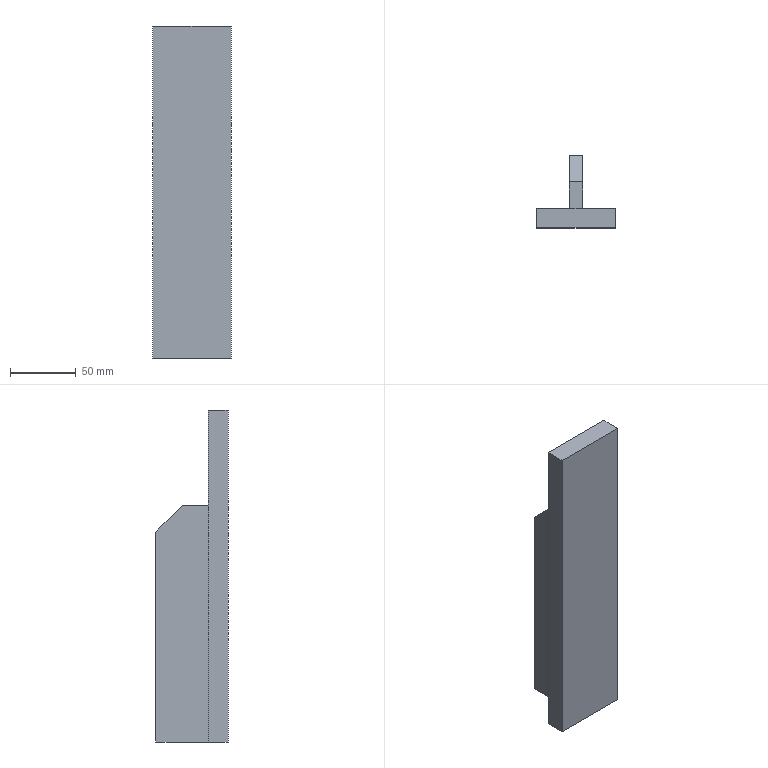Part | NX | features solid 2 | 1 solid | 11 faces | box 60 x 55 x 252.979 mm | volume 297681 mm3 | plane 11
STEP:
#1=CARTESIAN_POINT('',(-35.,-842.5,-290.));
#2=VERTEX_POINT('',#1);
#3=CARTESIAN_POINT('',(25.,-842.5,-290.));
#4=VERTEX_POINT('',#3);
#5=CARTESIAN_POINT('',(15.,-842.5,-290.));
#6=DIRECTION('',(1.,0.,0.));
#7=VECTOR('',#6,1000.);
#8=LINE('',#5,#7);
#9=EDGE_CURVE('',#2,#4,#8,.T.);
#10=ORIENTED_EDGE('',*,*,#9,.F.);
#11=CARTESIAN_POINT('',(-35.,-827.5,-290.));
#12=VERTEX_POINT('',#11);
#13=CARTESIAN_POINT('',(-35.,-842.5,-290.));
#14=DIRECTION('',(0.,-1.,0.));
#15=VECTOR('',#14,1000.);
#16=LINE('',#13,#15);
#17=EDGE_CURVE('',#12,#2,#16,.T.);
#18=ORIENTED_EDGE('',*,*,#17,.F.);
#19=CARTESIAN_POINT('',(-10.,-827.5,-290.));
#20=VERTEX_POINT('',#19);
#21=CARTESIAN_POINT('',(15.,-827.5,-290.));
#22=DIRECTION('',(1.,0.,0.));
#23=VECTOR('',#22,1000.);
#24=LINE('',#21,#23);
#25=EDGE_CURVE('',#12,#20,#24,.T.);
#26=ORIENTED_EDGE('',*,*,#25,.T.);
#27=CARTESIAN_POINT('',(-10.,-787.5,-290.));
#28=VERTEX_POINT('',#27);
#29=CARTESIAN_POINT('',(-10.,-827.5,-290.));
#30=DIRECTION('',(0.,1.,0.));
#31=VECTOR('',#30,1000.);
#32=LINE('',#29,#31);
#33=EDGE_CURVE('',#20,#28,#32,.T.);
#34=ORIENTED_EDGE('',*,*,#33,.T.);
#35=CARTESIAN_POINT('',(0.,-787.5,-290.));
#36=VERTEX_POINT('',#35);
#37=CARTESIAN_POINT('',(15.,-787.5,-290.));
#38=DIRECTION('',(1.,0.,0.));
#39=VECTOR('',#38,1000.);
#40=LINE('',#37,#39);
#41=EDGE_CURVE('',#28,#36,#40,.T.);
#42=ORIENTED_EDGE('',*,*,#41,.T.);
#43=CARTESIAN_POINT('',(0.,-827.5,-290.));
#44=VERTEX_POINT('',#43);
#45=CARTESIAN_POINT('',(0.,-827.5,-290.));
#46=DIRECTION('',(0.,1.,0.));
#47=VECTOR('',#46,1000.);
#48=LINE('',#45,#47);
#49=EDGE_CURVE('',#44,#36,#48,.T.);
#50=ORIENTED_EDGE('',*,*,#49,.F.);
#51=CARTESIAN_POINT('',(25.,-827.5,-290.));
#52=VERTEX_POINT('',#51);
#53=CARTESIAN_POINT('',(15.,-827.5,-290.));
#54=DIRECTION('',(1.,0.,0.));
#55=VECTOR('',#54,1000.);
#56=LINE('',#53,#55);
#57=EDGE_CURVE('',#44,#52,#56,.T.);
#58=ORIENTED_EDGE('',*,*,#57,.T.);
#59=CARTESIAN_POINT('',(25.,-835.,-290.));
#60=DIRECTION('',(0.,1.,0.));
#61=VECTOR('',#60,1000.);
#62=LINE('',#59,#61);
#63=EDGE_CURVE('',#52,#4,#62,.F.);
#64=ORIENTED_EDGE('',*,*,#63,.T.);
#65=EDGE_LOOP('',(#10,#18,#26,#34,#42,#50,#58,#64));
#66=FACE_BOUND('',#65,.T.);
#67=CARTESIAN_POINT('',(15.,-842.5,-290.));
#68=DIRECTION('',(0.,0.,-1.));
#69=DIRECTION('',(-1.,0.,0.));
#70=AXIS2_PLACEMENT_3D('',#67,#68,#69);
#71=PLANE('',#70);
#72=ADVANCED_FACE('',(#66),#71,.T.);
#73=CARTESIAN_POINT('',(-10.,-807.5,-110.));
#74=VERTEX_POINT('',#73);
#75=CARTESIAN_POINT('',(-10.,-787.5,-130.));
#76=VERTEX_POINT('',#75);
#77=CARTESIAN_POINT('',(-10.,-787.5,-130.));
#78=DIRECTION('',(0.,0.7071,-0.7071));
#79=VECTOR('',#78,1000.);
#80=LINE('',#77,#79);
#81=EDGE_CURVE('',#74,#76,#80,.T.);
#82=ORIENTED_EDGE('',*,*,#81,.F.);
#83=CARTESIAN_POINT('',(0.,-807.5,-110.));
#84=VERTEX_POINT('',#83);
#85=CARTESIAN_POINT('',(-5.,-807.5,-110.));
#86=DIRECTION('',(1.,0.,0.));
#87=VECTOR('',#86,1000.);
#88=LINE('',#85,#87);
#89=EDGE_CURVE('',#84,#74,#88,.F.);
#90=ORIENTED_EDGE('',*,*,#89,.F.);
#91=CARTESIAN_POINT('',(0.,-787.5,-130.));
#92=VERTEX_POINT('',#91);
#93=CARTESIAN_POINT('',(0.,-717.5,-200.));
#94=DIRECTION('',(0.,-0.7071,0.7071));
#95=VECTOR('',#94,1000.);
#96=LINE('',#93,#95);
#97=EDGE_CURVE('',#92,#84,#96,.T.);
#98=ORIENTED_EDGE('',*,*,#97,.F.);
#99=CARTESIAN_POINT('',(-5.,-787.5,-130.));
#100=DIRECTION('',(1.,0.,0.));
#101=VECTOR('',#100,1000.);
#102=LINE('',#99,#101);
#103=EDGE_CURVE('',#76,#92,#102,.T.);
#104=ORIENTED_EDGE('',*,*,#103,.F.);
#105=EDGE_LOOP('',(#82,#90,#98,#104));
#106=FACE_BOUND('',#105,.T.);
#107=CARTESIAN_POINT('',(-5.,-787.5,-130.));
#108=DIRECTION('',(0.,0.7071,0.7071));
#109=DIRECTION('',(0.,-0.7071,0.7071));
#110=AXIS2_PLACEMENT_3D('',#107,#108,#109);
#111=PLANE('',#110);
#112=ADVANCED_FACE('',(#106),#111,.T.);
#113=CARTESIAN_POINT('',(0.,-827.5,-110.));
#114=VERTEX_POINT('',#113);
#115=CARTESIAN_POINT('',(0.,-827.5,-110.));
#116=DIRECTION('',(0.,1.,0.));
#117=VECTOR('',#116,1000.);
#118=LINE('',#115,#117);
#119=EDGE_CURVE('',#114,#84,#118,.T.);
#120=ORIENTED_EDGE('',*,*,#119,.T.);
#121=ORIENTED_EDGE('',*,*,#89,.T.);
#122=CARTESIAN_POINT('',(-10.,-827.5,-110.));
#123=VERTEX_POINT('',#122);
#124=CARTESIAN_POINT('',(-10.,-827.5,-110.));
#125=DIRECTION('',(0.,1.,0.));
#126=VECTOR('',#125,1000.);
#127=LINE('',#124,#126);
#128=EDGE_CURVE('',#123,#74,#127,.T.);
#129=ORIENTED_EDGE('',*,*,#128,.F.);
#130=CARTESIAN_POINT('',(-5.,-827.5,-110.));
#131=DIRECTION('',(1.,0.,0.));
#132=VECTOR('',#131,1000.);
#133=LINE('',#130,#132);
#134=EDGE_CURVE('',#123,#114,#133,.T.);
#135=ORIENTED_EDGE('',*,*,#134,.T.);
#136=EDGE_LOOP('',(#120,#121,#129,#135));
#137=FACE_BOUND('',#136,.T.);
#138=CARTESIAN_POINT('',(-5.,-827.5,-110.));
#139=DIRECTION('',(0.,0.,-1.));
#140=DIRECTION('',(0.,1.,0.));
#141=AXIS2_PLACEMENT_3D('',#138,#139,#140);
#142=PLANE('',#141);
#143=ADVANCED_FACE('',(#137),#142,.F.);
#144=CARTESIAN_POINT('',(25.,-827.5,-37.021));
#145=VERTEX_POINT('',#144);
#146=CARTESIAN_POINT('',(-35.,-827.5,-37.021));
#147=VERTEX_POINT('',#146);
#148=CARTESIAN_POINT('',(-30.942,-827.5,-37.021));
#149=DIRECTION('',(-1.,0.,0.));
#150=VECTOR('',#149,1000.);
#151=LINE('',#148,#150);
#152=EDGE_CURVE('',#145,#147,#151,.T.);
#153=ORIENTED_EDGE('',*,*,#152,.F.);
#154=CARTESIAN_POINT('',(25.,-827.5,-51.379));
#155=DIRECTION('',(0.,0.,1.));
#156=VECTOR('',#155,1000.);
#157=LINE('',#154,#156);
#158=EDGE_CURVE('',#145,#52,#157,.F.);
#159=ORIENTED_EDGE('',*,*,#158,.T.);
#160=ORIENTED_EDGE('',*,*,#57,.F.);
#161=CARTESIAN_POINT('',(0.,-827.5,-310.));
#162=DIRECTION('',(0.,0.,1.));
#163=VECTOR('',#162,1000.);
#164=LINE('',#161,#163);
#165=EDGE_CURVE('',#44,#114,#164,.T.);
#166=ORIENTED_EDGE('',*,*,#165,.T.);
#167=ORIENTED_EDGE('',*,*,#134,.F.);
#168=CARTESIAN_POINT('',(-10.,-827.5,-310.));
#169=DIRECTION('',(0.,0.,1.));
#170=VECTOR('',#169,1000.);
#171=LINE('',#168,#170);
#172=EDGE_CURVE('',#20,#123,#171,.T.);
#173=ORIENTED_EDGE('',*,*,#172,.F.);
#174=ORIENTED_EDGE('',*,*,#25,.F.);
#175=CARTESIAN_POINT('',(-35.,-827.5,-21.795));
#176=DIRECTION('',(0.,0.,-1.));
#177=VECTOR('',#176,1000.);
#178=LINE('',#175,#177);
#179=EDGE_CURVE('',#147,#12,#178,.T.);
#180=ORIENTED_EDGE('',*,*,#179,.F.);
#181=EDGE_LOOP('',(#153,#159,#160,#166,#167,#173,#174,#180));
#182=FACE_BOUND('',#181,.T.);
#183=CARTESIAN_POINT('',(-30.942,-827.5,-21.795));
#184=DIRECTION('',(0.,1.,0.));
#185=DIRECTION('',(-1.,0.,0.));
#186=AXIS2_PLACEMENT_3D('',#183,#184,#185);
#187=PLANE('',#186);
#188=ADVANCED_FACE('',(#182),#187,.T.);
#189=CARTESIAN_POINT('',(0.,-787.5,-310.));
#190=DIRECTION('',(0.,0.,1.));
#191=VECTOR('',#190,1000.);
#192=LINE('',#189,#191);
#193=EDGE_CURVE('',#36,#92,#192,.T.);
#194=ORIENTED_EDGE('',*,*,#193,.T.);
#195=ORIENTED_EDGE('',*,*,#97,.T.);
#196=ORIENTED_EDGE('',*,*,#119,.F.);
#197=ORIENTED_EDGE('',*,*,#165,.F.);
#198=ORIENTED_EDGE('',*,*,#49,.T.);
#199=EDGE_LOOP('',(#194,#195,#196,#197,#198));
#200=FACE_BOUND('',#199,.T.);
#201=CARTESIAN_POINT('',(0.,-827.5,-310.));
#202=DIRECTION('',(1.,0.,0.));
#203=DIRECTION('',(0.,1.,0.));
#204=AXIS2_PLACEMENT_3D('',#201,#202,#203);
#205=PLANE('',#204);
#206=ADVANCED_FACE('',(#200),#205,.T.);
#207=CARTESIAN_POINT('',(-10.,-787.5,-310.));
#208=DIRECTION('',(0.,0.,1.));
#209=VECTOR('',#208,1000.);
#210=LINE('',#207,#209);
#211=EDGE_CURVE('',#28,#76,#210,.T.);
#212=ORIENTED_EDGE('',*,*,#211,.T.);
#213=ORIENTED_EDGE('',*,*,#103,.T.);
#214=ORIENTED_EDGE('',*,*,#193,.F.);
#215=ORIENTED_EDGE('',*,*,#41,.F.);
#216=EDGE_LOOP('',(#212,#213,#214,#215));
#217=FACE_BOUND('',#216,.T.);
#218=CARTESIAN_POINT('',(-5.,-787.5,-310.));
#219=DIRECTION('',(0.,1.,0.));
#220=DIRECTION('',(0.,0.,1.));
#221=AXIS2_PLACEMENT_3D('',#218,#219,#220);
#222=PLANE('',#221);
#223=ADVANCED_FACE('',(#217),#222,.T.);
#224=ORIENTED_EDGE('',*,*,#128,.T.);
#225=ORIENTED_EDGE('',*,*,#81,.T.);
#226=ORIENTED_EDGE('',*,*,#211,.F.);
#227=ORIENTED_EDGE('',*,*,#33,.F.);
#228=ORIENTED_EDGE('',*,*,#172,.T.);
#229=EDGE_LOOP('',(#224,#225,#226,#227,#228));
#230=FACE_BOUND('',#229,.T.);
#231=CARTESIAN_POINT('',(-10.,-827.5,-310.));
#232=DIRECTION('',(1.,0.,0.));
#233=DIRECTION('',(0.,1.,0.));
#234=AXIS2_PLACEMENT_3D('',#231,#232,#233);
#235=PLANE('',#234);
#236=ADVANCED_FACE('',(#230),#235,.F.);
#237=CARTESIAN_POINT('',(-35.,-842.5,-37.021));
#238=VERTEX_POINT('',#237);
#239=CARTESIAN_POINT('',(-35.,-842.5,-21.795));
#240=DIRECTION('',(0.,0.,-1.));
#241=VECTOR('',#240,1000.);
#242=LINE('',#239,#241);
#243=EDGE_CURVE('',#238,#2,#242,.T.);
#244=ORIENTED_EDGE('',*,*,#243,.F.);
#245=CARTESIAN_POINT('',(-35.,-835.,-37.021));
#246=DIRECTION('',(0.,1.,0.));
#247=VECTOR('',#246,1000.);
#248=LINE('',#245,#247);
#249=EDGE_CURVE('',#238,#147,#248,.T.);
#250=ORIENTED_EDGE('',*,*,#249,.T.);
#251=ORIENTED_EDGE('',*,*,#179,.T.);
#252=ORIENTED_EDGE('',*,*,#17,.T.);
#253=EDGE_LOOP('',(#244,#250,#251,#252));
#254=FACE_BOUND('',#253,.T.);
#255=CARTESIAN_POINT('',(-35.,-835.,-21.795));
#256=DIRECTION('',(1.,0.,0.));
#257=DIRECTION('',(0.,0.,-1.));
#258=AXIS2_PLACEMENT_3D('',#255,#256,#257);
#259=PLANE('',#258);
#260=ADVANCED_FACE('',(#254),#259,.F.);
#261=CARTESIAN_POINT('',(25.,-842.5,-37.021));
#262=VERTEX_POINT('',#261);
#263=CARTESIAN_POINT('',(25.,-842.5,-51.379));
#264=DIRECTION('',(0.,0.,1.));
#265=VECTOR('',#264,1000.);
#266=LINE('',#263,#265);
#267=EDGE_CURVE('',#262,#4,#266,.F.);
#268=ORIENTED_EDGE('',*,*,#267,.F.);
#269=CARTESIAN_POINT('',(-30.942,-842.5,-37.021));
#270=DIRECTION('',(-1.,0.,0.));
#271=VECTOR('',#270,1000.);
#272=LINE('',#269,#271);
#273=EDGE_CURVE('',#262,#238,#272,.T.);
#274=ORIENTED_EDGE('',*,*,#273,.T.);
#275=ORIENTED_EDGE('',*,*,#243,.T.);
#276=ORIENTED_EDGE('',*,*,#9,.T.);
#277=EDGE_LOOP('',(#268,#274,#275,#276));
#278=FACE_BOUND('',#277,.T.);
#279=CARTESIAN_POINT('',(-30.942,-842.5,-21.795));
#280=DIRECTION('',(0.,1.,0.));
#281=DIRECTION('',(-1.,0.,0.));
#282=AXIS2_PLACEMENT_3D('',#279,#280,#281);
#283=PLANE('',#282);
#284=ADVANCED_FACE('',(#278),#283,.F.);
#285=ORIENTED_EDGE('',*,*,#158,.F.);
#286=CARTESIAN_POINT('',(25.,-835.,-37.021));
#287=DIRECTION('',(0.,1.,0.));
#288=VECTOR('',#287,1000.);
#289=LINE('',#286,#288);
#290=EDGE_CURVE('',#145,#262,#289,.F.);
#291=ORIENTED_EDGE('',*,*,#290,.T.);
#292=ORIENTED_EDGE('',*,*,#267,.T.);
#293=ORIENTED_EDGE('',*,*,#63,.F.);
#294=EDGE_LOOP('',(#285,#291,#292,#293));
#295=FACE_BOUND('',#294,.T.);
#296=CARTESIAN_POINT('',(25.,-835.,-51.379));
#297=DIRECTION('',(1.,0.,0.));
#298=DIRECTION('',(0.,0.,-1.));
#299=AXIS2_PLACEMENT_3D('',#296,#297,#298);
#300=PLANE('',#299);
#301=ADVANCED_FACE('',(#295),#300,.T.);
#302=ORIENTED_EDGE('',*,*,#152,.T.);
#303=ORIENTED_EDGE('',*,*,#249,.F.);
#304=ORIENTED_EDGE('',*,*,#273,.F.);
#305=ORIENTED_EDGE('',*,*,#290,.F.);
#306=EDGE_LOOP('',(#302,#303,#304,#305));
#307=FACE_BOUND('',#306,.T.);
#308=CARTESIAN_POINT('',(14.128,-885.,-37.021));
#309=DIRECTION('',(0.,0.,-1.));
#310=DIRECTION('',(-1.,0.,0.));
#311=AXIS2_PLACEMENT_3D('',#308,#309,#310);
#312=PLANE('',#311);
#313=ADVANCED_FACE('',(#307),#312,.F.);
#314=CLOSED_SHELL('',(#72,#112,#143,#188,#206,#223,#236,#260,#284,#301,#313));
#315=MANIFOLD_SOLID_BREP('',#314);
#316=(LENGTH_UNIT()NAMED_UNIT(*)SI_UNIT(.MILLI.,.METRE.));
#317=UNCERTAINTY_MEASURE_WITH_UNIT(LENGTH_MEASURE(0.00001),#316,'','');
#318=(NAMED_UNIT(*)PLANE_ANGLE_UNIT()SI_UNIT($,.RADIAN.));
#319=(NAMED_UNIT(*)SI_UNIT($,.STERADIAN.)SOLID_ANGLE_UNIT());
#320=(GEOMETRIC_REPRESENTATION_CONTEXT(3)GLOBAL_UNCERTAINTY_ASSIGNED_CONTEXT((#317))GLOBAL_UNIT_ASSIGNED_CONTEXT((#316,#318,#319))REPRESENTATION_CONTEXT('',''));
#321=ADVANCED_BREP_SHAPE_REPRESENTATION('',(#315),#320);